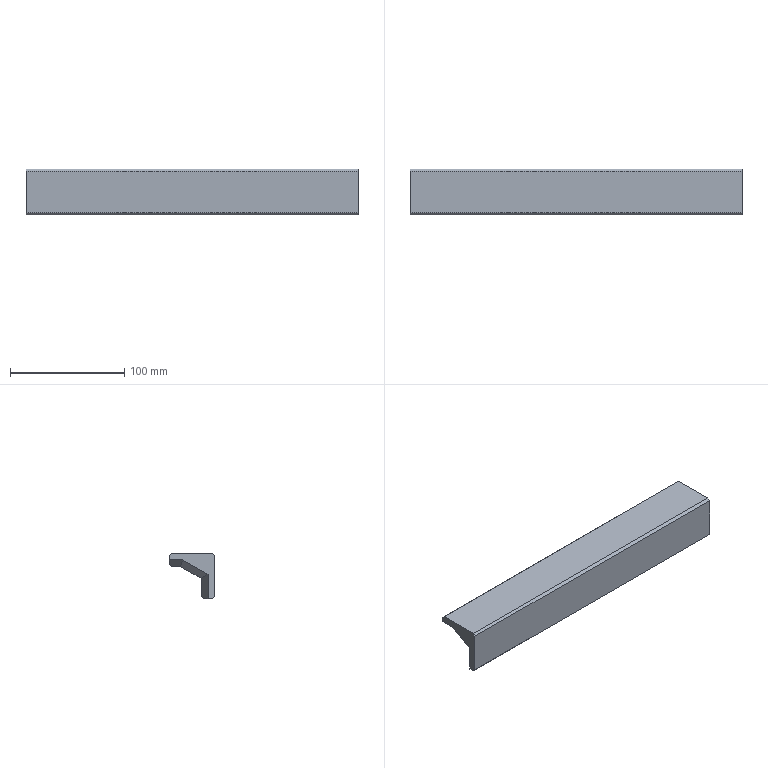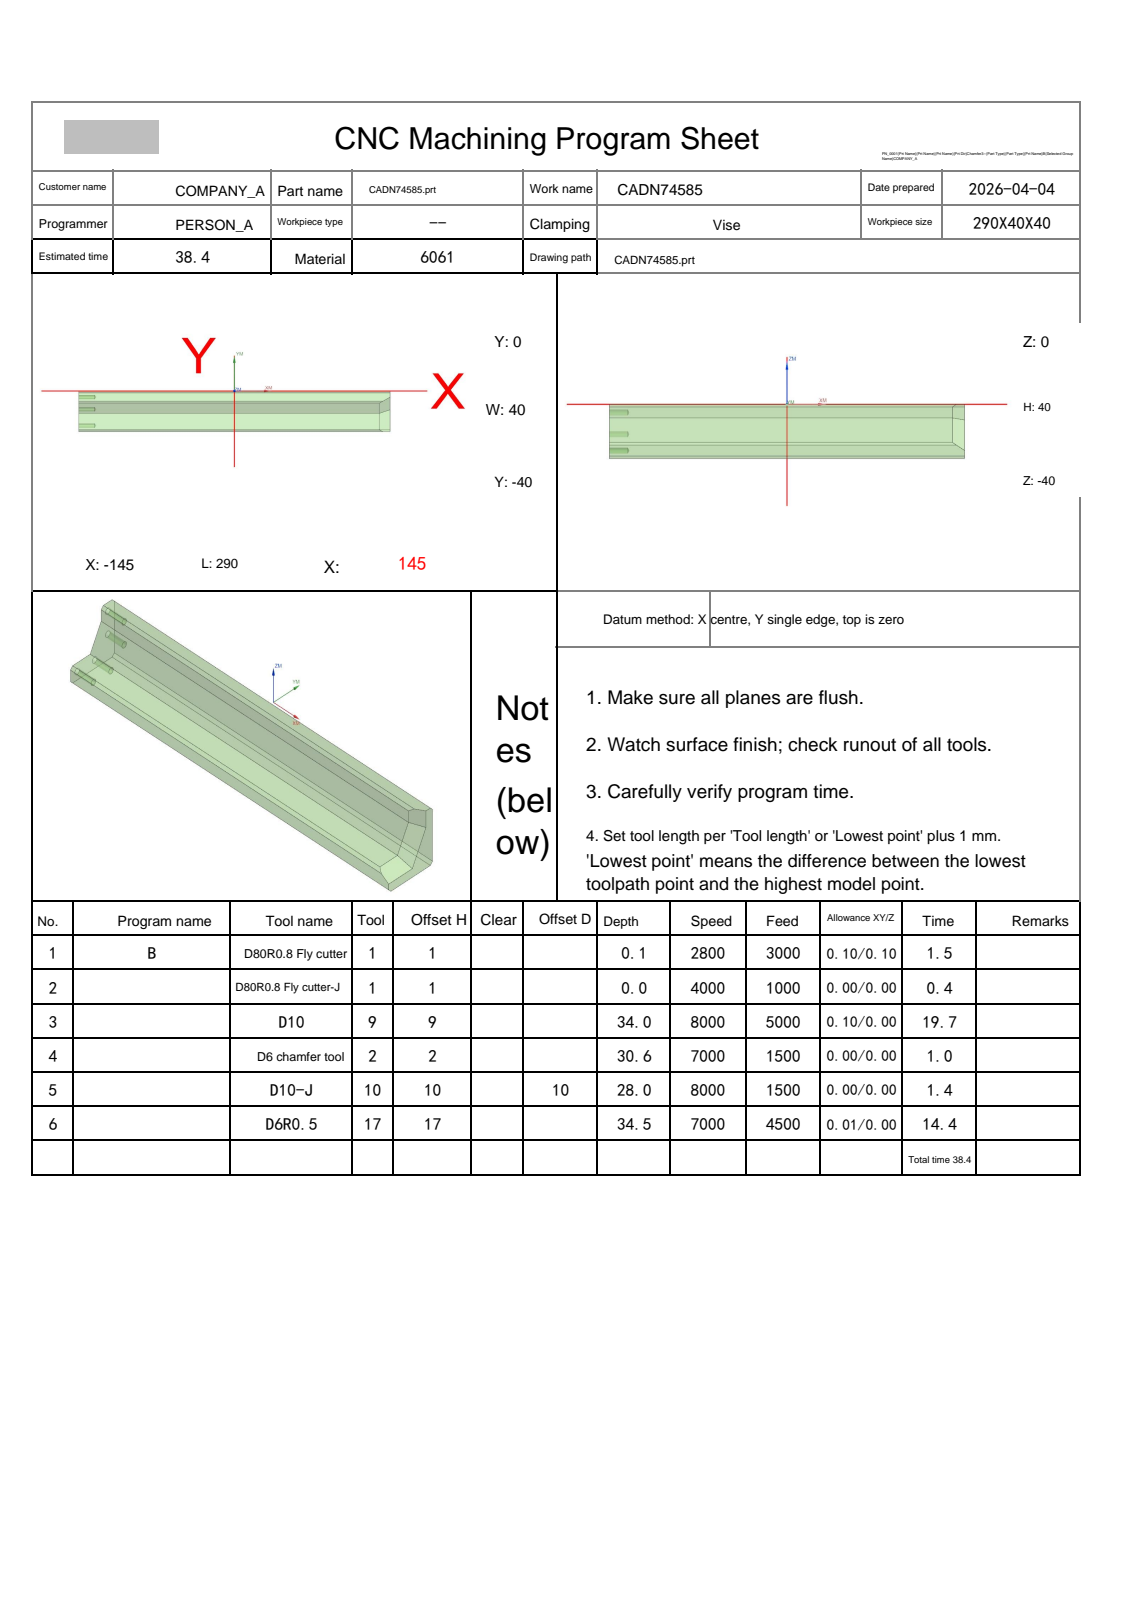NC program | NX | posted by the shop | part box 290 x 40 x 40 mm
Lines 1 to 109 of 6846:
%
O0001
(Machine time: 39.61 MIN)
(===Total Tool:5===)
(T1=D80R0.8 FlyCutter D=80.  R=0.8  D-  H01 Z=0.    )
(T9=D10     D=10.  R=0.   D-  H09 Z=-34.  )
(T2=D6Chamfer   D=6.   R=0.   D-  H02 Z=-30.6 )
(T10=D10-J  D=10.  R=0.   D10 H10 Z=-28.  )
(T17=D6R0.5 D=6.   R=0.5  D-  H17 Z=-34.5 )
G80 G90 G17 G49 G40
G91 G28 Z0
M01
N1 T01 M06
(D80R0.8 FlyCutter D=80. R=0.8 H=01 ce=0.10 di=0.10)
G00 G90 G54 X-197.097 Y-20. M03 S2800
G43 H01 Z20.
M08
Z6.011
G01 Z4.011 F3000.
X-185.097
X185.097
X197.097
Z6.011
G00 X-197.097
Z5.522
G01 Z3.522
X-185.097
X185.097
X197.097
Z5.522
G00 X-197.097
Z5.033
G01 Z3.033
X-185.097
X185.097
X197.097
Z5.033
G00 X-197.097
Z4.544
G01 Z2.544
X-185.097
X185.097
X197.097
Z4.544
G00 Z20.
X-197.097
Z4.056
G01 Z2.056
X-185.097
X185.097
X197.097
Z4.056
G00 Z20.
X-197.097
Z3.567
G01 Z1.567
X-185.097
X185.097
X197.097
Z3.567
G00 Z20.
X-197.097
Z3.078
G01 Z1.078
X-185.097
X185.097
X197.097
Z3.078
G00 Z20.
X-197.097
Z2.589
G01 Z.589
X-185.097
X185.097
X197.097
Z2.589
G00 Z20.
X-197.097
Z2.1
G01 Z.1
X-185.097
X185.097
X197.097
Z2.1
G00 Z20.
G91 G28 Z0.0
M05
M09
G91 G28 Z0.0
M01
N2 T01 M06
(D80R0.8 FlyCutter-J D=80. R=0.8 H=01 ce=0.00 di=0.00)
G00 G90 G54 X-196.999 Y-20. M03 S4000
G43 H01 Z20.
M08
Z2.
G01 Z0.0 F1000.
X-184.999
X184.999
X196.999
Z2.
G00 Z20.
G91 G28 Z0.0
M05
M09
G91 G28 Z0.0
M01